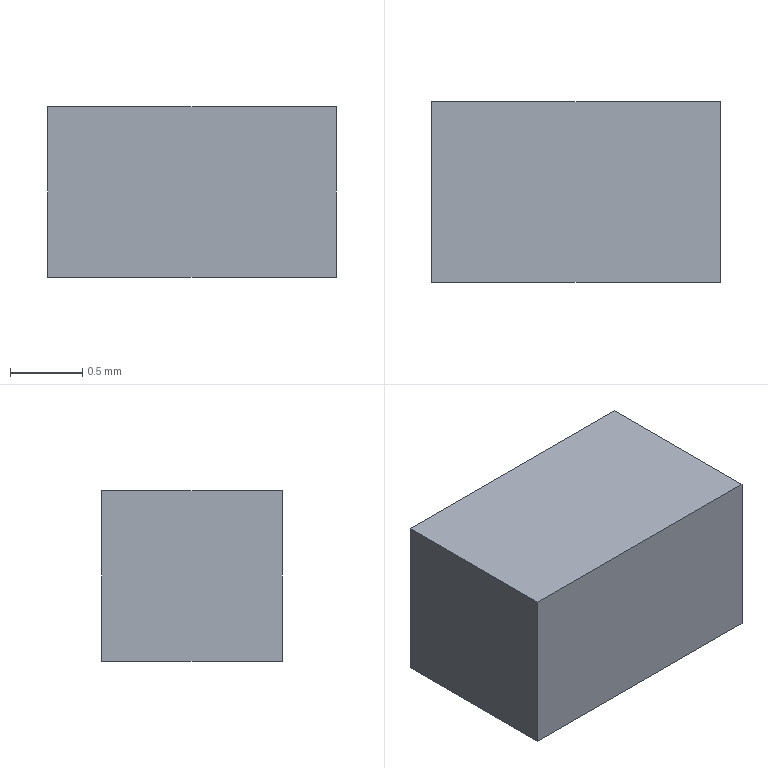Part | Creo | 1 solid | 6 faces | box 2 x 1.25 x 1.179 mm | volume 2.948 mm3 | plane 6
STEP:
#1=CARTESIAN_POINT('',(0.,0.,0.));
#2=DIRECTION('',(0.,0.,1.));
#3=DIRECTION('',(1.,0.,0.));
#4=AXIS2_PLACEMENT_3D('',#1,#2,#3);
#5=CARTESIAN_POINT('',(-1.,0.625,0.));
#6=VERTEX_POINT('',#5);
#7=CARTESIAN_POINT('',(-1.,-0.625,0.));
#8=VERTEX_POINT('',#7);
#9=CARTESIAN_POINT('',(-1.,0.625,0.));
#10=DIRECTION('',(0.,-1.,0.));
#11=VECTOR('',#10,1.25);
#12=LINE('',#9,#11);
#13=EDGE_CURVE('',#6,#8,#12,.T.);
#14=ORIENTED_EDGE('',*,*,#13,.T.);
#15=CARTESIAN_POINT('',(1.,-0.625,0.));
#16=VERTEX_POINT('',#15);
#17=CARTESIAN_POINT('',(-1.,-0.625,0.));
#18=DIRECTION('',(1.,0.,0.));
#19=VECTOR('',#18,2.);
#20=LINE('',#17,#19);
#21=EDGE_CURVE('',#8,#16,#20,.T.);
#22=ORIENTED_EDGE('',*,*,#21,.T.);
#23=CARTESIAN_POINT('',(1.,0.625,0.));
#24=VERTEX_POINT('',#23);
#25=CARTESIAN_POINT('',(1.,-0.625,0.));
#26=DIRECTION('',(0.,1.,0.));
#27=VECTOR('',#26,1.25);
#28=LINE('',#25,#27);
#29=EDGE_CURVE('',#16,#24,#28,.T.);
#30=ORIENTED_EDGE('',*,*,#29,.T.);
#31=CARTESIAN_POINT('',(1.,0.625,0.));
#32=DIRECTION('',(-1.,0.,0.));
#33=VECTOR('',#32,2.);
#34=LINE('',#31,#33);
#35=EDGE_CURVE('',#24,#6,#34,.T.);
#36=ORIENTED_EDGE('',*,*,#35,.T.);
#37=EDGE_LOOP('',(#14,#22,#30,#36));
#38=FACE_OUTER_BOUND('',#37,.F.);
#39=CARTESIAN_POINT('',(0.,0.,0.));
#40=DIRECTION('',(0.,0.,1.));
#41=DIRECTION('',(1.,0.,0.));
#42=AXIS2_PLACEMENT_3D('',#39,#40,#41);
#43=PLANE('',#42);
#44=ADVANCED_FACE('',(#38),#43,.F.);
#45=ORIENTED_EDGE('',*,*,#13,.F.);
#46=CARTESIAN_POINT('',(-1.,0.625,1.179));
#47=VERTEX_POINT('',#46);
#48=CARTESIAN_POINT('',(-1.,0.625,0.));
#49=DIRECTION('',(0.,0.,1.));
#50=VECTOR('',#49,1.179);
#51=LINE('',#48,#50);
#52=EDGE_CURVE('',#6,#47,#51,.T.);
#53=ORIENTED_EDGE('',*,*,#52,.T.);
#54=CARTESIAN_POINT('',(-1.,-0.625,1.179));
#55=VERTEX_POINT('',#54);
#56=CARTESIAN_POINT('',(-1.,0.625,1.179));
#57=DIRECTION('',(0.,-1.,0.));
#58=VECTOR('',#57,1.25);
#59=LINE('',#56,#58);
#60=EDGE_CURVE('',#47,#55,#59,.T.);
#61=ORIENTED_EDGE('',*,*,#60,.T.);
#62=CARTESIAN_POINT('',(-1.,-0.625,0.));
#63=DIRECTION('',(0.,0.,1.));
#64=VECTOR('',#63,1.179);
#65=LINE('',#62,#64);
#66=EDGE_CURVE('',#8,#55,#65,.T.);
#67=ORIENTED_EDGE('',*,*,#66,.F.);
#68=EDGE_LOOP('',(#45,#53,#61,#67));
#69=FACE_OUTER_BOUND('',#68,.F.);
#70=CARTESIAN_POINT('',(-1.,0.625,0.));
#71=DIRECTION('',(-1.,0.,0.));
#72=DIRECTION('',(0.,-1.,0.));
#73=AXIS2_PLACEMENT_3D('',#70,#71,#72);
#74=PLANE('',#73);
#75=ADVANCED_FACE('',(#69),#74,.T.);
#76=ORIENTED_EDGE('',*,*,#35,.F.);
#77=CARTESIAN_POINT('',(1.,0.625,1.179));
#78=VERTEX_POINT('',#77);
#79=CARTESIAN_POINT('',(1.,0.625,0.));
#80=DIRECTION('',(0.,0.,1.));
#81=VECTOR('',#80,1.179);
#82=LINE('',#79,#81);
#83=EDGE_CURVE('',#24,#78,#82,.T.);
#84=ORIENTED_EDGE('',*,*,#83,.T.);
#85=CARTESIAN_POINT('',(1.,0.625,1.179));
#86=DIRECTION('',(-1.,0.,0.));
#87=VECTOR('',#86,2.);
#88=LINE('',#85,#87);
#89=EDGE_CURVE('',#78,#47,#88,.T.);
#90=ORIENTED_EDGE('',*,*,#89,.T.);
#91=ORIENTED_EDGE('',*,*,#52,.F.);
#92=EDGE_LOOP('',(#76,#84,#90,#91));
#93=FACE_OUTER_BOUND('',#92,.F.);
#94=CARTESIAN_POINT('',(1.,0.625,0.));
#95=DIRECTION('',(0.,1.,0.));
#96=DIRECTION('',(-1.,0.,0.));
#97=AXIS2_PLACEMENT_3D('',#94,#95,#96);
#98=PLANE('',#97);
#99=ADVANCED_FACE('',(#93),#98,.T.);
#100=ORIENTED_EDGE('',*,*,#29,.F.);
#101=CARTESIAN_POINT('',(1.,-0.625,1.179));
#102=VERTEX_POINT('',#101);
#103=CARTESIAN_POINT('',(1.,-0.625,0.));
#104=DIRECTION('',(0.,0.,1.));
#105=VECTOR('',#104,1.179);
#106=LINE('',#103,#105);
#107=EDGE_CURVE('',#16,#102,#106,.T.);
#108=ORIENTED_EDGE('',*,*,#107,.T.);
#109=CARTESIAN_POINT('',(1.,-0.625,1.179));
#110=DIRECTION('',(0.,1.,0.));
#111=VECTOR('',#110,1.25);
#112=LINE('',#109,#111);
#113=EDGE_CURVE('',#102,#78,#112,.T.);
#114=ORIENTED_EDGE('',*,*,#113,.T.);
#115=ORIENTED_EDGE('',*,*,#83,.F.);
#116=EDGE_LOOP('',(#100,#108,#114,#115));
#117=FACE_OUTER_BOUND('',#116,.F.);
#118=CARTESIAN_POINT('',(1.,-0.625,0.));
#119=DIRECTION('',(1.,0.,0.));
#120=DIRECTION('',(0.,1.,0.));
#121=AXIS2_PLACEMENT_3D('',#118,#119,#120);
#122=PLANE('',#121);
#123=ADVANCED_FACE('',(#117),#122,.T.);
#124=ORIENTED_EDGE('',*,*,#21,.F.);
#125=ORIENTED_EDGE('',*,*,#66,.T.);
#126=CARTESIAN_POINT('',(-1.,-0.625,1.179));
#127=DIRECTION('',(1.,0.,0.));
#128=VECTOR('',#127,2.);
#129=LINE('',#126,#128);
#130=EDGE_CURVE('',#55,#102,#129,.T.);
#131=ORIENTED_EDGE('',*,*,#130,.T.);
#132=ORIENTED_EDGE('',*,*,#107,.F.);
#133=EDGE_LOOP('',(#124,#125,#131,#132));
#134=FACE_OUTER_BOUND('',#133,.F.);
#135=CARTESIAN_POINT('',(-1.,-0.625,0.));
#136=DIRECTION('',(0.,-1.,0.));
#137=DIRECTION('',(1.,0.,0.));
#138=AXIS2_PLACEMENT_3D('',#135,#136,#137);
#139=PLANE('',#138);
#140=ADVANCED_FACE('',(#134),#139,.T.);
#141=ORIENTED_EDGE('',*,*,#60,.F.);
#142=ORIENTED_EDGE('',*,*,#89,.F.);
#143=ORIENTED_EDGE('',*,*,#113,.F.);
#144=ORIENTED_EDGE('',*,*,#130,.F.);
#145=EDGE_LOOP('',(#141,#142,#143,#144));
#146=FACE_OUTER_BOUND('',#145,.F.);
#147=CARTESIAN_POINT('',(0.,0.,1.179));
#148=DIRECTION('',(0.,0.,1.));
#149=DIRECTION('',(1.,0.,0.));
#150=AXIS2_PLACEMENT_3D('',#147,#148,#149);
#151=PLANE('',#150);
#152=ADVANCED_FACE('',(#146),#151,.T.);
#153=CLOSED_SHELL('',(#44,#75,#99,#123,#140,#152));
#154=MANIFOLD_SOLID_BREP('',#153);
#155=(LENGTH_UNIT()NAMED_UNIT(*)SI_UNIT(.MILLI.,.METRE.));
#156=UNCERTAINTY_MEASURE_WITH_UNIT(LENGTH_MEASURE(0.0002637),#155,'','');
#157=(NAMED_UNIT(*)PLANE_ANGLE_UNIT()SI_UNIT($,.RADIAN.));
#158=PLANE_ANGLE_MEASURE_WITH_UNIT(PLANE_ANGLE_MEASURE(0.01745),#157);
#159=(CONVERSION_BASED_UNIT('DEGREE',#158)NAMED_UNIT(*)PLANE_ANGLE_UNIT());
#160=(NAMED_UNIT(*)SI_UNIT($,.STERADIAN.)SOLID_ANGLE_UNIT());
#161=(GEOMETRIC_REPRESENTATION_CONTEXT(3)GLOBAL_UNCERTAINTY_ASSIGNED_CONTEXT((#156))GLOBAL_UNIT_ASSIGNED_CONTEXT((#155,#159,#160))REPRESENTATION_CONTEXT('',''));
#162=ADVANCED_BREP_SHAPE_REPRESENTATION('',(#4,#154),#161);